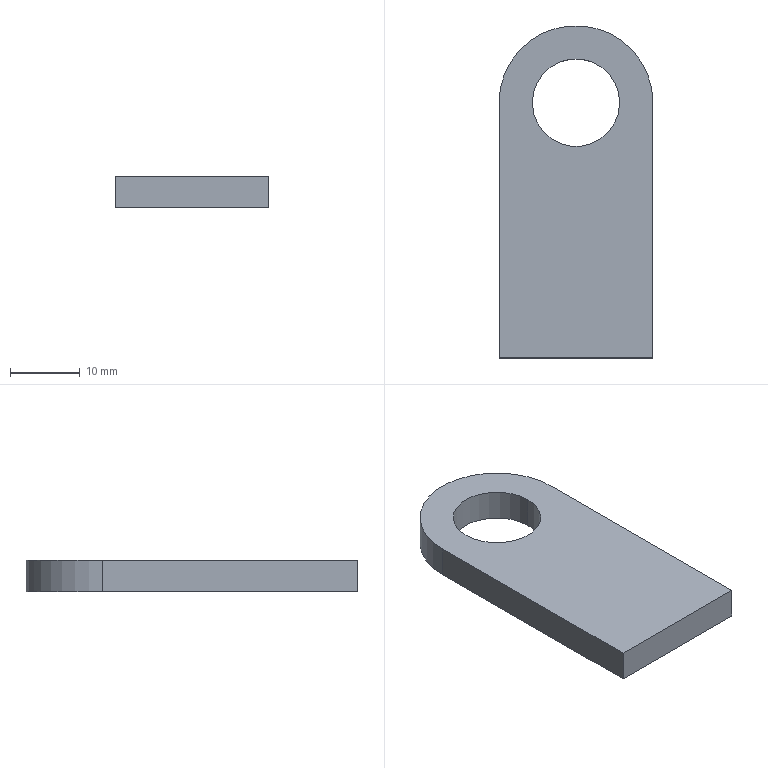Part | SolidWorks | features FlatPattern 1, SMBaseFlange 1, SheetMetal 1 | 1 solid | 8 faces | box 22 x 47.5 x 4.5 mm | volume 3917 mm3 | plane 5 | cylinder 3 | commonest cylinder face diameters 12.5 x2 22 x1
STEP:
#1=CARTESIAN_POINT('',(-6.25,0.,4.5));
#2=VERTEX_POINT('',#1);
#3=CARTESIAN_POINT('',(6.25,0.,4.5));
#4=VERTEX_POINT('',#3);
#5=CARTESIAN_POINT('',(0.,0.,4.5));
#6=DIRECTION('',(0.,0.,1.));
#7=DIRECTION('',(1.,0.,0.));
#8=AXIS2_PLACEMENT_3D('',#5,#6,#7);
#9=CIRCLE('',#8,6.25);
#10=EDGE_CURVE('',#2,#4,#9,.T.);
#11=ORIENTED_EDGE('',*,*,#10,.T.);
#12=CARTESIAN_POINT('',(6.25,0.,0.));
#13=VERTEX_POINT('',#12);
#14=CARTESIAN_POINT('',(6.25,0.,4.5));
#15=DIRECTION('',(0.,0.,-1.));
#16=VECTOR('',#15,1000.);
#17=LINE('',#14,#16);
#18=EDGE_CURVE('',#4,#13,#17,.T.);
#19=ORIENTED_EDGE('',*,*,#18,.T.);
#20=CARTESIAN_POINT('',(-6.25,0.,0.));
#21=VERTEX_POINT('',#20);
#22=CARTESIAN_POINT('',(0.,0.,0.));
#23=DIRECTION('',(0.,0.,1.));
#24=DIRECTION('',(1.,0.,0.));
#25=AXIS2_PLACEMENT_3D('',#22,#23,#24);
#26=CIRCLE('',#25,6.25);
#27=EDGE_CURVE('',#21,#13,#26,.T.);
#28=ORIENTED_EDGE('',*,*,#27,.F.);
#29=CARTESIAN_POINT('',(-6.25,0.,4.5));
#30=DIRECTION('',(0.,0.,-1.));
#31=VECTOR('',#30,1000.);
#32=LINE('',#29,#31);
#33=EDGE_CURVE('',#2,#21,#32,.T.);
#34=ORIENTED_EDGE('',*,*,#33,.F.);
#35=EDGE_LOOP('',(#11,#19,#28,#34));
#36=FACE_OUTER_BOUND('',#35,.T.);
#37=CARTESIAN_POINT('',(0.,0.,4.5));
#38=DIRECTION('',(0.,0.,-1.));
#39=DIRECTION('',(-1.,0.,0.));
#40=AXIS2_PLACEMENT_3D('',#37,#38,#39);
#41=CYLINDRICAL_SURFACE('',#40,6.25);
#42=ADVANCED_FACE('',(#36),#41,.F.);
#43=CARTESIAN_POINT('',(11.,0.,4.5));
#44=VERTEX_POINT('',#43);
#45=CARTESIAN_POINT('',(-11.,0.,4.5));
#46=VERTEX_POINT('',#45);
#47=CARTESIAN_POINT('',(0.,0.,4.5));
#48=DIRECTION('',(0.,0.,1.));
#49=DIRECTION('',(1.,0.,0.));
#50=AXIS2_PLACEMENT_3D('',#47,#48,#49);
#51=CIRCLE('',#50,11.);
#52=EDGE_CURVE('',#44,#46,#51,.T.);
#53=ORIENTED_EDGE('',*,*,#52,.T.);
#54=CARTESIAN_POINT('',(-11.,-36.5,4.5));
#55=VERTEX_POINT('',#54);
#56=CARTESIAN_POINT('',(-11.,0.,4.5));
#57=DIRECTION('',(0.,-1.,0.));
#58=VECTOR('',#57,1000.);
#59=LINE('',#56,#58);
#60=EDGE_CURVE('',#46,#55,#59,.T.);
#61=ORIENTED_EDGE('',*,*,#60,.T.);
#62=CARTESIAN_POINT('',(11.,-36.5,4.5));
#63=VERTEX_POINT('',#62);
#64=CARTESIAN_POINT('',(-11.,-36.5,4.5));
#65=DIRECTION('',(1.,0.,0.));
#66=VECTOR('',#65,1000.);
#67=LINE('',#64,#66);
#68=EDGE_CURVE('',#55,#63,#67,.T.);
#69=ORIENTED_EDGE('',*,*,#68,.T.);
#70=CARTESIAN_POINT('',(11.,-36.5,4.5));
#71=DIRECTION('',(0.,1.,0.));
#72=VECTOR('',#71,1000.);
#73=LINE('',#70,#72);
#74=EDGE_CURVE('',#63,#44,#73,.T.);
#75=ORIENTED_EDGE('',*,*,#74,.T.);
#76=EDGE_LOOP('',(#53,#61,#69,#75));
#77=FACE_OUTER_BOUND('',#76,.T.);
#78=ORIENTED_EDGE('',*,*,#10,.F.);
#79=CARTESIAN_POINT('',(0.,0.,4.5));
#80=DIRECTION('',(0.,0.,1.));
#81=DIRECTION('',(1.,0.,0.));
#82=AXIS2_PLACEMENT_3D('',#79,#80,#81);
#83=CIRCLE('',#82,6.25);
#84=EDGE_CURVE('',#4,#2,#83,.T.);
#85=ORIENTED_EDGE('',*,*,#84,.F.);
#86=EDGE_LOOP('',(#78,#85));
#87=FACE_BOUND('',#86,.T.);
#88=CARTESIAN_POINT('',(0.,0.,4.5));
#89=DIRECTION('',(0.,0.,1.));
#90=DIRECTION('',(1.,0.,0.));
#91=AXIS2_PLACEMENT_3D('',#88,#89,#90);
#92=PLANE('',#91);
#93=ADVANCED_FACE('',(#77,#87),#92,.T.);
#94=CARTESIAN_POINT('',(11.,0.,0.));
#95=VERTEX_POINT('',#94);
#96=CARTESIAN_POINT('',(-11.,0.,0.));
#97=VERTEX_POINT('',#96);
#98=CARTESIAN_POINT('',(0.,0.,0.));
#99=DIRECTION('',(0.,0.,1.));
#100=DIRECTION('',(1.,0.,0.));
#101=AXIS2_PLACEMENT_3D('',#98,#99,#100);
#102=CIRCLE('',#101,11.);
#103=EDGE_CURVE('',#95,#97,#102,.T.);
#104=ORIENTED_EDGE('',*,*,#103,.F.);
#105=CARTESIAN_POINT('',(11.,-36.5,0.));
#106=VERTEX_POINT('',#105);
#107=CARTESIAN_POINT('',(11.,-36.5,0.));
#108=DIRECTION('',(0.,1.,0.));
#109=VECTOR('',#108,1000.);
#110=LINE('',#107,#109);
#111=EDGE_CURVE('',#106,#95,#110,.T.);
#112=ORIENTED_EDGE('',*,*,#111,.F.);
#113=CARTESIAN_POINT('',(-11.,-36.5,0.));
#114=VERTEX_POINT('',#113);
#115=CARTESIAN_POINT('',(-11.,-36.5,0.));
#116=DIRECTION('',(1.,0.,0.));
#117=VECTOR('',#116,1000.);
#118=LINE('',#115,#117);
#119=EDGE_CURVE('',#114,#106,#118,.T.);
#120=ORIENTED_EDGE('',*,*,#119,.F.);
#121=CARTESIAN_POINT('',(-11.,0.,0.));
#122=DIRECTION('',(0.,-1.,0.));
#123=VECTOR('',#122,1000.);
#124=LINE('',#121,#123);
#125=EDGE_CURVE('',#97,#114,#124,.T.);
#126=ORIENTED_EDGE('',*,*,#125,.F.);
#127=EDGE_LOOP('',(#104,#112,#120,#126));
#128=FACE_OUTER_BOUND('',#127,.T.);
#129=ORIENTED_EDGE('',*,*,#27,.T.);
#130=CARTESIAN_POINT('',(0.,0.,0.));
#131=DIRECTION('',(0.,0.,1.));
#132=DIRECTION('',(1.,0.,0.));
#133=AXIS2_PLACEMENT_3D('',#130,#131,#132);
#134=CIRCLE('',#133,6.25);
#135=EDGE_CURVE('',#13,#21,#134,.T.);
#136=ORIENTED_EDGE('',*,*,#135,.T.);
#137=EDGE_LOOP('',(#129,#136));
#138=FACE_BOUND('',#137,.T.);
#139=CARTESIAN_POINT('',(0.,0.,0.));
#140=DIRECTION('',(0.,0.,1.));
#141=DIRECTION('',(1.,0.,0.));
#142=AXIS2_PLACEMENT_3D('',#139,#140,#141);
#143=PLANE('',#142);
#144=ADVANCED_FACE('',(#128,#138),#143,.F.);
#145=ORIENTED_EDGE('',*,*,#103,.T.);
#146=CARTESIAN_POINT('',(-11.,0.,4.5));
#147=DIRECTION('',(0.,0.,-1.));
#148=VECTOR('',#147,1000.);
#149=LINE('',#146,#148);
#150=EDGE_CURVE('',#46,#97,#149,.T.);
#151=ORIENTED_EDGE('',*,*,#150,.F.);
#152=ORIENTED_EDGE('',*,*,#52,.F.);
#153=CARTESIAN_POINT('',(11.,0.,4.5));
#154=DIRECTION('',(0.,0.,-1.));
#155=VECTOR('',#154,1000.);
#156=LINE('',#153,#155);
#157=EDGE_CURVE('',#44,#95,#156,.T.);
#158=ORIENTED_EDGE('',*,*,#157,.T.);
#159=EDGE_LOOP('',(#145,#151,#152,#158));
#160=FACE_OUTER_BOUND('',#159,.T.);
#161=CARTESIAN_POINT('',(0.,0.,4.5));
#162=DIRECTION('',(0.,0.,-1.));
#163=DIRECTION('',(-1.,0.,0.));
#164=AXIS2_PLACEMENT_3D('',#161,#162,#163);
#165=CYLINDRICAL_SURFACE('',#164,11.);
#166=ADVANCED_FACE('',(#160),#165,.T.);
#167=ORIENTED_EDGE('',*,*,#125,.T.);
#168=CARTESIAN_POINT('',(-11.,-36.5,4.5));
#169=DIRECTION('',(0.,0.,-1.));
#170=VECTOR('',#169,1000.);
#171=LINE('',#168,#170);
#172=EDGE_CURVE('',#55,#114,#171,.T.);
#173=ORIENTED_EDGE('',*,*,#172,.F.);
#174=ORIENTED_EDGE('',*,*,#60,.F.);
#175=ORIENTED_EDGE('',*,*,#150,.T.);
#176=EDGE_LOOP('',(#167,#173,#174,#175));
#177=FACE_OUTER_BOUND('',#176,.T.);
#178=CARTESIAN_POINT('',(-11.,0.,4.5));
#179=DIRECTION('',(1.,0.,0.));
#180=DIRECTION('',(0.,1.,0.));
#181=AXIS2_PLACEMENT_3D('',#178,#179,#180);
#182=PLANE('',#181);
#183=ADVANCED_FACE('',(#177),#182,.F.);
#184=ORIENTED_EDGE('',*,*,#119,.T.);
#185=CARTESIAN_POINT('',(11.,-36.5,4.5));
#186=DIRECTION('',(0.,0.,-1.));
#187=VECTOR('',#186,1000.);
#188=LINE('',#185,#187);
#189=EDGE_CURVE('',#63,#106,#188,.T.);
#190=ORIENTED_EDGE('',*,*,#189,.F.);
#191=ORIENTED_EDGE('',*,*,#68,.F.);
#192=ORIENTED_EDGE('',*,*,#172,.T.);
#193=EDGE_LOOP('',(#184,#190,#191,#192));
#194=FACE_OUTER_BOUND('',#193,.T.);
#195=CARTESIAN_POINT('',(-11.,-36.5,4.5));
#196=DIRECTION('',(0.,1.,0.));
#197=DIRECTION('',(0.,0.,1.));
#198=AXIS2_PLACEMENT_3D('',#195,#196,#197);
#199=PLANE('',#198);
#200=ADVANCED_FACE('',(#194),#199,.F.);
#201=ORIENTED_EDGE('',*,*,#111,.T.);
#202=ORIENTED_EDGE('',*,*,#157,.F.);
#203=ORIENTED_EDGE('',*,*,#74,.F.);
#204=ORIENTED_EDGE('',*,*,#189,.T.);
#205=EDGE_LOOP('',(#201,#202,#203,#204));
#206=FACE_OUTER_BOUND('',#205,.T.);
#207=CARTESIAN_POINT('',(11.,-36.5,4.5));
#208=DIRECTION('',(-1.,0.,0.));
#209=DIRECTION('',(0.,-1.,0.));
#210=AXIS2_PLACEMENT_3D('',#207,#208,#209);
#211=PLANE('',#210);
#212=ADVANCED_FACE('',(#206),#211,.F.);
#213=ORIENTED_EDGE('',*,*,#18,.F.);
#214=ORIENTED_EDGE('',*,*,#84,.T.);
#215=ORIENTED_EDGE('',*,*,#33,.T.);
#216=ORIENTED_EDGE('',*,*,#135,.F.);
#217=EDGE_LOOP('',(#213,#214,#215,#216));
#218=FACE_OUTER_BOUND('',#217,.T.);
#219=CARTESIAN_POINT('',(0.,0.,4.5));
#220=DIRECTION('',(0.,0.,-1.));
#221=DIRECTION('',(-1.,0.,0.));
#222=AXIS2_PLACEMENT_3D('',#219,#220,#221);
#223=CYLINDRICAL_SURFACE('',#222,6.25);
#224=ADVANCED_FACE('',(#218),#223,.F.);
#225=CLOSED_SHELL('',(#42,#93,#144,#166,#183,#200,#212,#224));
#226=MANIFOLD_SOLID_BREP('',#225);
#227=CARTESIAN_POINT('',(0.,0.,0.));
#228=DIRECTION('',(0.,0.,1.));
#229=DIRECTION('',(1.,0.,0.));
#230=AXIS2_PLACEMENT_3D('',#227,#228,#229);
#231=(LENGTH_UNIT()NAMED_UNIT(*)SI_UNIT(.MILLI.,.METRE.));
#232=UNCERTAINTY_MEASURE_WITH_UNIT(LENGTH_MEASURE(0.00001),#231,'','');
#233=(NAMED_UNIT(*)PLANE_ANGLE_UNIT()SI_UNIT($,.RADIAN.));
#234=(NAMED_UNIT(*)SI_UNIT($,.STERADIAN.)SOLID_ANGLE_UNIT());
#235=(GEOMETRIC_REPRESENTATION_CONTEXT(3)GLOBAL_UNCERTAINTY_ASSIGNED_CONTEXT((#232))GLOBAL_UNIT_ASSIGNED_CONTEXT((#231,#233,#234))REPRESENTATION_CONTEXT('',''));
#236=ADVANCED_BREP_SHAPE_REPRESENTATION('',(#226,#230),#235);